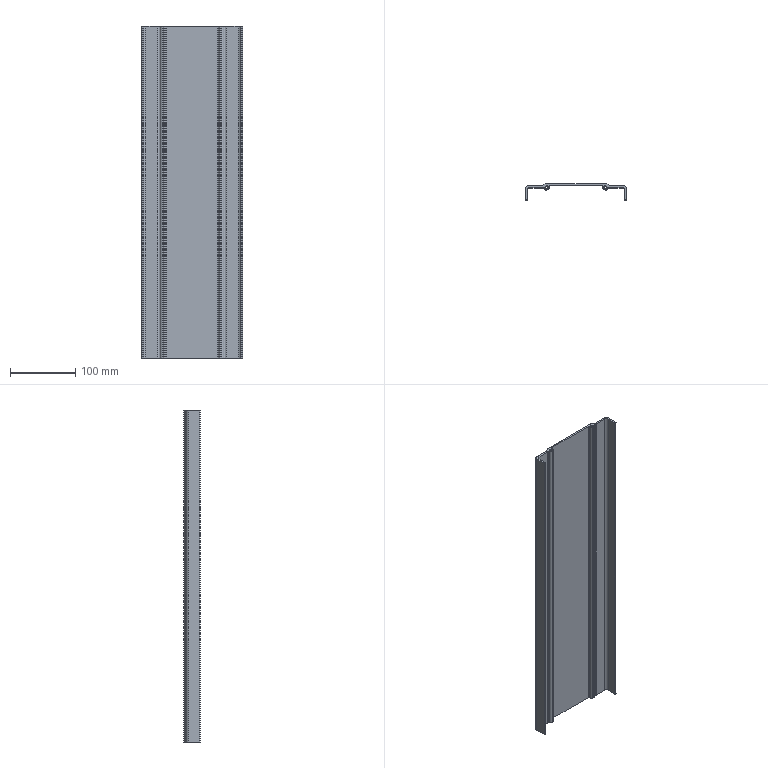Part | STEP file | 1 solid | 52 faces | box 155 x 25 x 509.4 mm | volume 278478 mm3 | cylinder 32 | plane 20 | commonest cylinder face diameters 8 x14 1 x12 3 x4 4.2 x2